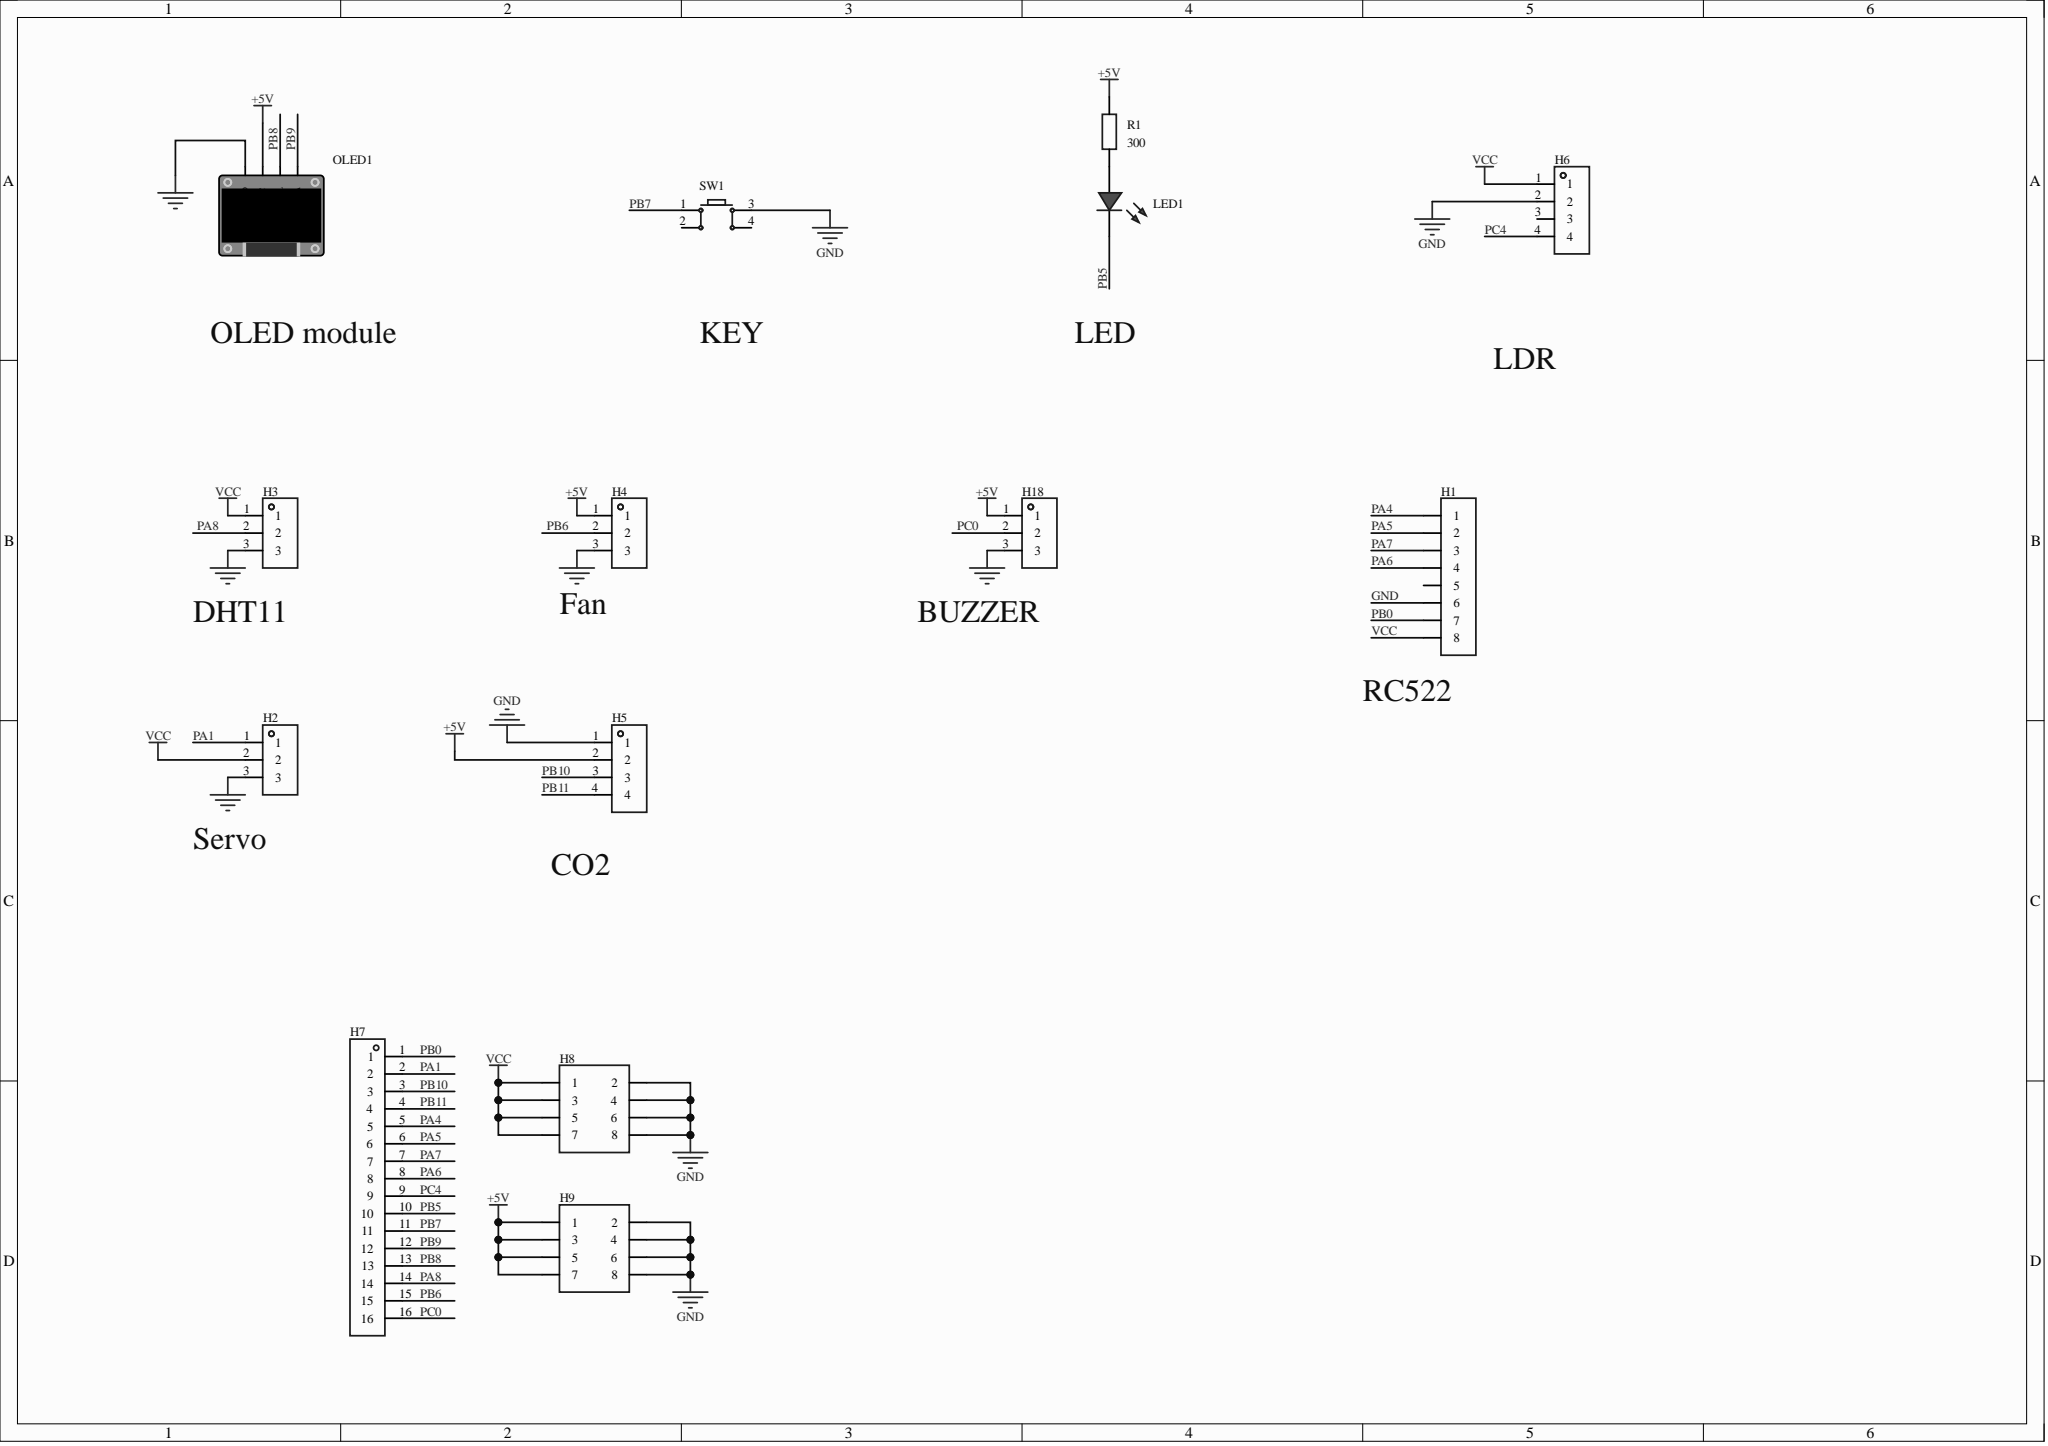Circuit board | Altium Designer | 14 parts | 20 nets
Bill of materials:
Comment,Description,Designator,Footprint,LibRef,Quantity
"","","H1","HDR-TH_8P-P2.54-V-F-1","HDR-F_2.54_1x8P","1"
"","","H2, H3, H4, H18","HDR-TH_3P-P2.54-V-F","HDR-F_2.54_1x3P","4"
"","","H5, H6","HDR-TH_4P-P2.54-V-F","HDR-F_2.54_1x4P","2"
"","","H7","HDR-TH_16P-P2.54-V-F","HDR-F_2.54_1x16P","1"
"","","H8, H9","HDR-TH_8P-P2.54-V-F-R2-C4-S2.54-1","HDR-F_2.54_2x4","2"
"","","LED1","LED_TH-3mm","LED_TH-R_3mm","1"
"","","OLED1","0.96OLED_4P","0.96OLED模块_4P","1"
"300","","R1","Res_1/8W","Res_AXIAL-1/8W","1"
"","","SW1","SW-TH_4P-L6.0-W6.0-P4.50-LS6.5","Key_TH_6x6x6","1"
Netlist (Protel format):
[
H1
HDR-TH_8P-P2.54-V-F-1




]
[
H2
HDR-TH_3P-P2.54-V-F




]
[
H3
HDR-TH_3P-P2.54-V-F




]
[
H4
HDR-TH_3P-P2.54-V-F




]
[
H5
HDR-TH_4P-P2.54-V-F




]
[
H6
HDR-TH_4P-P2.54-V-F




]
[
H7
HDR-TH_16P-P2.54-V-F




]
[
H8
HDR-TH_8P-P2.54-V-F-R2-C4-S2.54-1




]
[
H9
HDR-TH_8P-P2.54-V-F-R2-C4-S2.54-1




]
[
H18
HDR-TH_3P-P2.54-V-F




]
[
LED1
LED_TH-3mm




]
[
OLED1
0.96OLED_4P




]
[
R1
Res_1/8W
300



]
[
SW1
SW-TH_4P-L6.0-W6.0-P4.50-LS6.5




]
(
VCC
H1-8
H2-2
H3-1
H6-1
H8-1
H8-3
H8-5
H8-7
)
(
PC4
H6-4
H7-9
)
(
PC0
H7-16
H18-2
)
(
PB11
H5-4
H7-4
)
(
PB10
H5-3
H7-3
)
(
PB9
H7-12
OLED1-4
)
(
PB8
H7-13
OLED1-3
)
(
PB7
H7-11
SW1-1
)
(
PB6
H4-2
H7-15
)
(
PB5
H7-10
LED1-2
)
(
PB0
H1-7
H7-1
)
(
PA8
H3-2
H7-14
)
(
PA7
H1-3
H7-7
)
(
PA6
H1-4
H7-8
)
(
PA5
H1-2
H7-6
)
(
PA4
H1-1
H7-5
)
(
PA1
H2-1
H7-2
)
(
NetLED1_1
LED1-1
R1-1
)
(
GND
H1-6
H2-3
H3-3
H4-3
H5-1
H6-2
H8-2
H8-4
H8-6
H8-8
H9-2
H9-4
H9-6
H9-8
H18-3
OLED1-1
SW1-3
)
(
+5V
H4-1
H5-2
H9-1
H9-3
H9-5
H9-7
H18-1
OLED1-2
R1-2
)